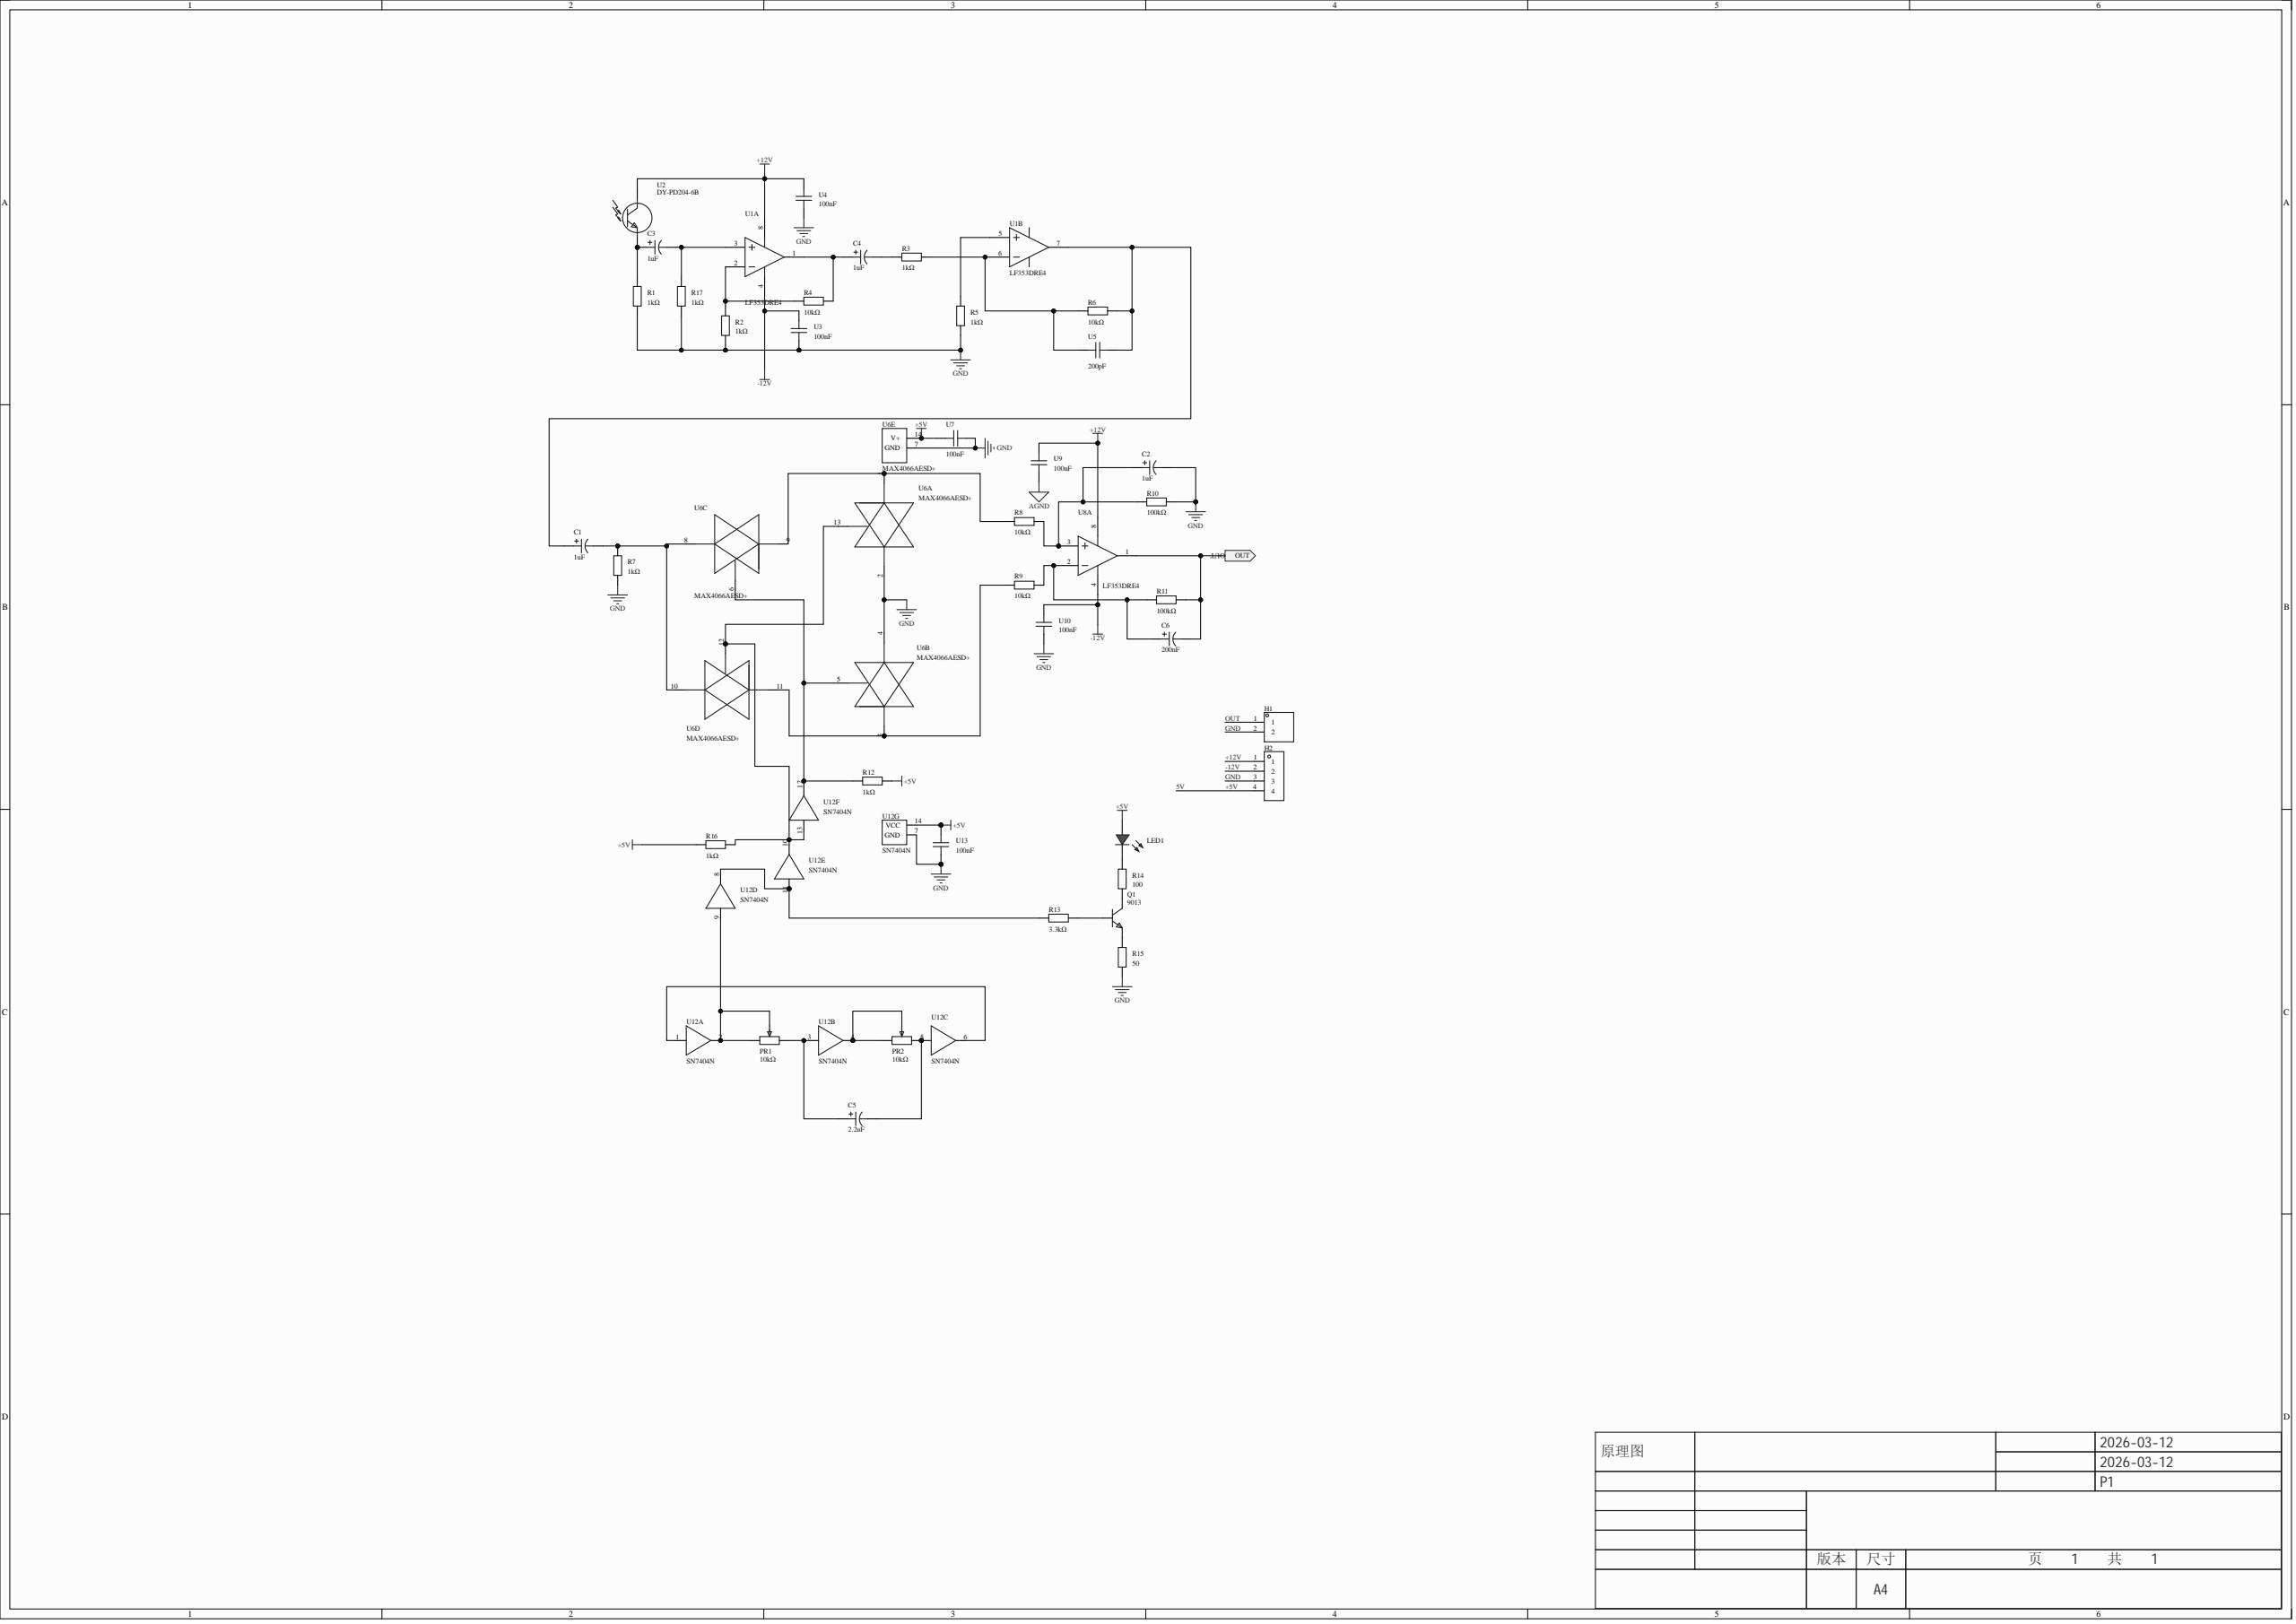Circuit board | Altium Designer | 41 parts | 30 nets
Bill of materials:
Comment,Description,Designator,Footprint,LibRef,Quantity
"1uF","","C1, C2, C3, C4","CAP-TH_BD6.3-P2.50-D0.5-FD","1uF450V6.3x12KM","4"
"2.2uF","","C5","CAP-TH_BD8.0-P3.50-D0.5-FD","2.2uF450V8x12KM","1"
"200nF","","C6","CAP-TH_BD6.3-P2.50-D0.5-FD","1uF450V6.3x12KM","1"
"","","H1","HDR-TH_2P-P2.54-V-M-1","HDR-M_2.54_1x2P","1"
"","","H2","HDR-TH_4P-P2.54-V-M","HDR-M_2.54_1x4P","1"
"","","LED1","LED_TH-3mm","LED_TH-R_3mm","1"
"10kΩ","","PR1, PR2","R_3296","R_3296","2"
"9013","晶体管类型:NPN;集电极电流(Ic):500mA;集射极击穿电压(Vceo):20V;耗散功率(Pd):625mW;直流电流增益(hFE):276@50mA,1.0V;","Q1","TO-92-3_L4.8-W3.7-P2.54-R","9013","1"
"1kΩ","","R1, R2, R3, R5, R7, R12, R16, R17","Res_1/8W","Res_AXIAL-1/8W","8"
"10kΩ","","R4, R6, R8, R9","Res_1/8W","Res_AXIAL-1/8W","4"
"100kΩ","","R10, R11","Res_1/8W","Res_AXIAL-1/8W","2"
"3.3kΩ","","R13","Res_1/8W","Res_AXIAL-1/8W","1"
"100","","R14","Res_1/8W","Res_AXIAL-1/8W","1"
"50","","R15","Res_1/8W","Res_AXIAL-1/8W","1"
"LF353DRE4","增益带宽积(GBP):3MHz;输入偏置电流(Ib):50pA;输入失调电压(Vos):5mV;压摆率(SR):13V/us;","U1, U8","SOIC-8_L5.0-W4.0-P1.27-LS6.1-BL","LF353DRE4","2"
"DY-PD204-6B","DY-PD204-6B 是一种 NPN 型高速度和高敏感的光敏二极管。","U2","LED-TH_BD3.0-P2.54-FD","DY-PD204-6B","1"
"100nF","","U3, U4, U7, U9, U10, U13","CAP-TH_L5.0-W2.5-P5.00-D1.0","100nF","6"
"200pF","容值:200pF;精度:±5%;额定电压:100V;温度系数:-;","U5","CAP-TH_L4.9-W3.7-P5.08-D0.5","CC4-0805-CG-100V-200PF-J","1"
"MAX4066AESD+","","U6","SOIC-14_L8.7-W3.9-P1.27-LS6.0-BL","MAX4066AESD+","1"
"SN7404N","SN7404 6 通道、4.75V 至 5.25V 双极反相器","U12","PDIP-14_L19.3-W6.4-P2.54-LS7.9-BL-1","SN7404N","1"
Netlist (Protel format):
[
C1
CAP-TH_BD6.3-P2.50-D0.5-FD
1uF



]
[
C2
CAP-TH_BD6.3-P2.50-D0.5-FD
1uF



]
[
C3
CAP-TH_BD6.3-P2.50-D0.5-FD
1uF



]
[
C4
CAP-TH_BD6.3-P2.50-D0.5-FD
1uF



]
[
C5
CAP-TH_BD8.0-P3.50-D0.5-FD
2.2uF



]
[
C6
CAP-TH_BD6.3-P2.50-D0.5-FD
200nF



]
[
H1
HDR-TH_2P-P2.54-V-M-1




]
[
H2
HDR-TH_4P-P2.54-V-M




]
[
LED1
LED_TH-3mm




]
[
PR1
R_3296
10kΩ



]
[
PR2
R_3296
10kΩ



]
[
Q1
TO-92-3_L4.8-W3.7-P2.54-R
9013



]
[
R1
Res_1/8W
1kΩ



]
[
R2
Res_1/8W
1kΩ



]
[
R3
Res_1/8W
1kΩ



]
[
R4
Res_1/8W
10kΩ



]
[
R5
Res_1/8W
1kΩ



]
[
R6
Res_1/8W
10kΩ



]
[
R7
Res_1/8W
1kΩ



]
[
R8
Res_1/8W
10kΩ



]
[
R9
Res_1/8W
10kΩ



]
[
R10
Res_1/8W
100kΩ



]
[
R11
Res_1/8W
100kΩ



]
[
R12
Res_1/8W
1kΩ



]
[
R13
Res_1/8W
3.3kΩ



]
[
R14
Res_1/8W
100



]
[
R15
Res_1/8W
50



]
[
R16
Res_1/8W
1kΩ



]
[
R17
Res_1/8W
1kΩ



]
[
U1
SOIC-8_L5.0-W4.0-P1.27-LS6.1-BL
LF353DRE4



]
[
U2
LED-TH_BD3.0-P2.54-FD
DY-PD204-6B



]
[
U3
CAP-TH_L5.0-W2.5-P5.00-D1.0
100nF



]
[
U4
CAP-TH_L5.0-W2.5-P5.00-D1.0
100nF



]
[
U5
CAP-TH_L4.9-W3.7-P5.08-D0.5
200pF



]
[
U6
SOIC-14_L8.7-W3.9-P1.27-LS6.0-BL
MAX4066AESD+



]
[
U7
CAP-TH_L5.0-W2.5-P5.00-D1.0
100nF



]
[
U8
SOIC-8_L5.0-W4.0-P1.27-LS6.1-BL
LF353DRE4



]
[
U9
CAP-TH_L5.0-W2.5-P5.00-D1.0
100nF



]
[
U10
CAP-TH_L5.0-W2.5-P5.00-D1.0
100nF



]
[
U12
PDIP-14_L19.3-W6.4-P2.54-LS7.9-BL-1
SN7404N



]
[
U13
CAP-TH_L5.0-W2.5-P5.00-D1.0
100nF



]
(
OUT
C6-2
H1-1
R11-2
U8-1
)
(
NetU12_1
U12-1
U12-6
)
(
NetR16_2
R16-2
U6-12
U6-13
U12-10
U12-13
)
(
NetR13_1
R13-1
U12-8
U12-11
)
(
NetR12_2
R12-2
U6-5
U6-6
U12-12
)
(
NetR9_1
R9-1
U6-3
U6-11
)
(
NetR8_1
R8-1
U6-1
U6-9
)
(
NetR5_1
R5-1
U1-5
)
(
NetR3_1
R3-1
R6-1
U1-6
U5-1
)
(
NetR2_2
R2-2
R4-1
U1-2
)
(
NetQ1_3
Q1-3
R15-2
)
(
NetQ1_2
Q1-2
R13-2
)
(
NetQ1_1
Q1-1
R14-1
)
(
NetPR2_2
PR2-2
PR2-3
U12-4
)
(
NetPR1_2
PR1-2
PR1-3
U12-2
U12-9
)
(
NetLED1_2
LED1-2
R14-2
)
(
NetC6_1
C6-1
R9-2
R11-1
U8-2
)
(
NetC5_2
C5-2
PR2-1
U12-5
)
(
NetC5_1
C5-1
PR1-1
U12-3
)
(
NetC4_2
C4-2
R3-2
)
(
NetC4_1
C4-1
R4-2
U1-1
)
(
NetC3_2
C3-2
R17-2
U1-3
)
(
NetC3_1
C3-1
R1-2
U2-1
)
(
NetC2_1
C2-1
R8-2
R10-1
U8-3
)
(
NetC1_2
C1-2
R7-2
U6-8
U6-10
)
(
NetC1_1
C1-1
R6-2
U1-7
U5-2
)
(
GND
C2-2
H1-2
H2-3
R1-1
R2-1
R5-2
R7-1
R10-2
R15-1
R17-1
U3-2
U4-2
U6-2
U6-4
U6-7
U7-2
U10-1
U12-7
U13-1
)
(
-12V
H2-2
U1-4
U3-1
U8-4
U10-2
)
(
+12V
H2-1
U1-8
U2-2
U4-1
U8-8
U9-2
)
(
5V
H2-4
LED1-1
R12-1
R16-1
U6-14
U7-1
U12-14
U13-2
)